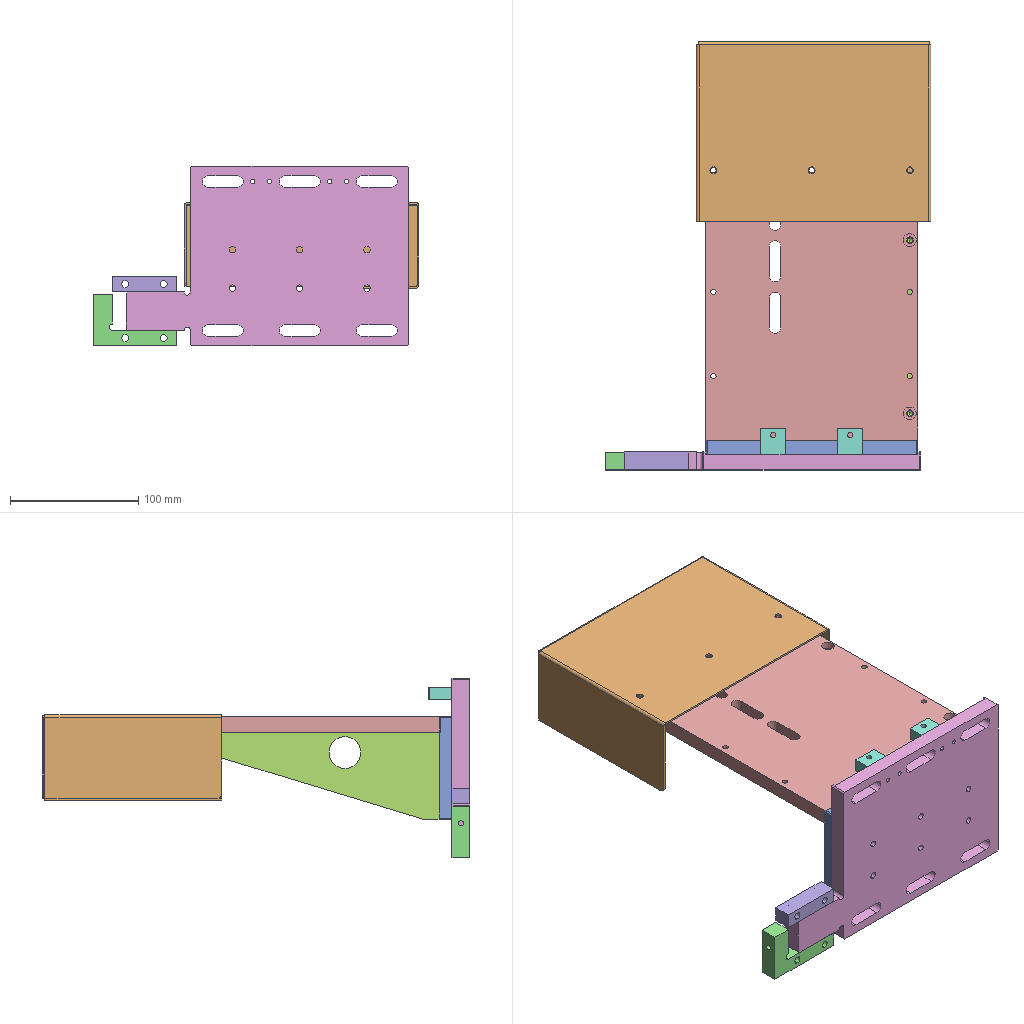Assembly | SolidWorks | 9 different items | 10 placed | box 254 x 333 x 140 mm
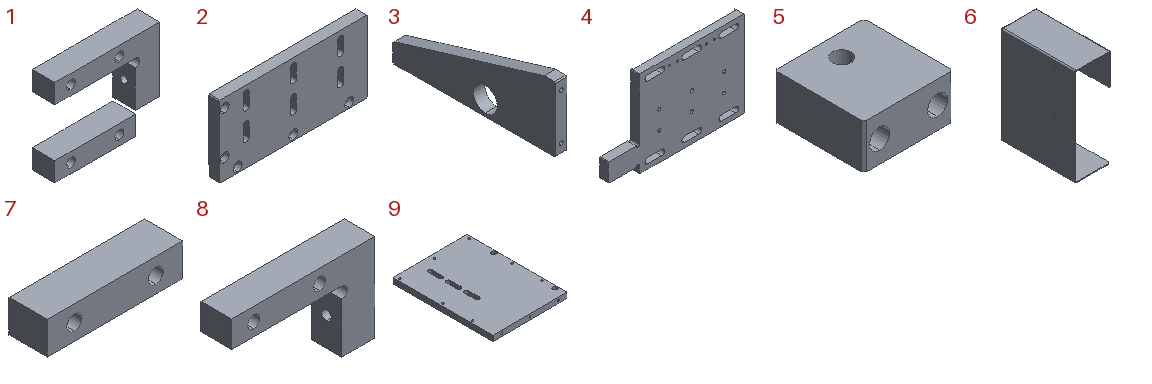Parts list (item | name | quantity | parent item | size | volume | features):
1 | (subassembly) | x1 | - | 65 x 14 x 54 mm | 22275 mm3 | -
2 | - | x1 | - | 165 x 12 x 80 mm | 144651 mm3 | features HoleWzd 3, Chamfer 1, Extrusion 1, ICE 1
3 | - | x1 | - | 12 x 170 x 68 mm | 86588 mm3 | features HoleWzd 2, Chamfer 1, Extrusion 1, ICE 1
4 | - | x1 | - | 220 x 14 x 140 mm | 286346 mm3 | features HoleWzd 3, ICE 3, Chamfer 1, Extrusion 1
5 | - | x2 | - | 20 x 20 x 10 mm | 3220 mm3 | features HoleWzd 2, Chamfer 1, Extrusion 1
6 | - | x1 | - | 66.5 x 140 x 183 mm | 93527 mm3 | features EdgeFlange 2, Fillet 1, FlatPattern 1, HoleWzd 1, SMBaseFlange 1, SheetMetal 1
7 | - | x1 | in 1 | 50 x 14 x 12 mm | 7110 mm3 | features Extrusion 1, HoleWzd 1
8 | - | x1 | in 1 | 65 x 14 x 40 mm | 15165 mm3 | features HoleWzd 2, ICE 2, Extrusion 1
9 | - | x1 | - | 165 x 220.4 x 12 mm | 385919 mm3 | features HoleWzd 4, Chamfer 1, Extrusion 1, Fillet 1, ICE 1
Mates (type | each side: item.copy, entity, surface, feature):
In the top assembly
Coincident | 9.1 face plane Boss-Extrude1 | 2.1 face plane Cut-Extrude1
Coincident | 9.1 face plane Boss-Extrude1 | 2.1 face plane Boss-Extrude1
Width | 2.1 face plane Boss-Extrude1 | 2.1 face plane Boss-Extrude1 | 9.1 face plane Boss-Extrude1 | 9.1 face plane Boss-Extrude1
Coincident | 9.1 face plane Boss-Extrude1 | 3.1 face plane Boss-Extrude1 | 2 times
Coincident | 2.1 face plane Boss-Extrude1 | 3.1 face plane Boss-Extrude1
Coincident | 2.1 face plane Boss-Extrude1 | 4.1 face plane Cut-Extrude1 | 2 times
Width | 2.1 face plane Boss-Extrude1 | 2.1 face plane Boss-Extrude1 | 4.1 face plane Cut-Extrude1 | 4.1 face plane Cut-Extrude1
Width | 2.1 face plane Boss-Extrude1 | 2.1 face plane Boss-Extrude1 | 4.1 face plane Boss-Extrude1 | 4.1 face plane Boss-Extrude1
Coincident | 4.1 face plane Cut-Extrude1 | 5.1 face plane Boss-Extrude1
Concentric | 4.1 face cylinder M4 Tapped Hole1 | 5.1 face cylinder M4 Clearance Hole1 | 2 times
Concentric | 4.1 face cylinder M4 Tapped Hole1 | 5.2 face cylinder M4 Clearance Hole1 | 2 times
Coincident | 4.1 face plane Cut-Extrude1 | 5.2 face plane Boss-Extrude1
Coincident | 9.1 face plane Boss-Extrude1 | 6.1 face plane Base-Flange1
Concentric | 9.1 face cylinder M5 Tapped Hole2 | 6.1 face cylinder M5 Clearance Hole1 | 2 times
Coincident | 4.1 face plane Boss-Extrude1 | 8.1 face plane Boss-Extrude1
Coincident | 4.1 face plane Boss-Extrude2 | 8.1 face plane Boss-Extrude1
DistanceDim | 7.1 face plane Boss-Extrude1 | 4.1 face plane Boss-Extrude1
In subassembly 1
Coincident | 7.2 face plane Boss-Extrude1 | 8.2 face plane Boss-Extrude1 | 2 times
DistanceDim | 8.2 face plane Boss-Extrude1 | 7.2 face plane Boss-Extrude1